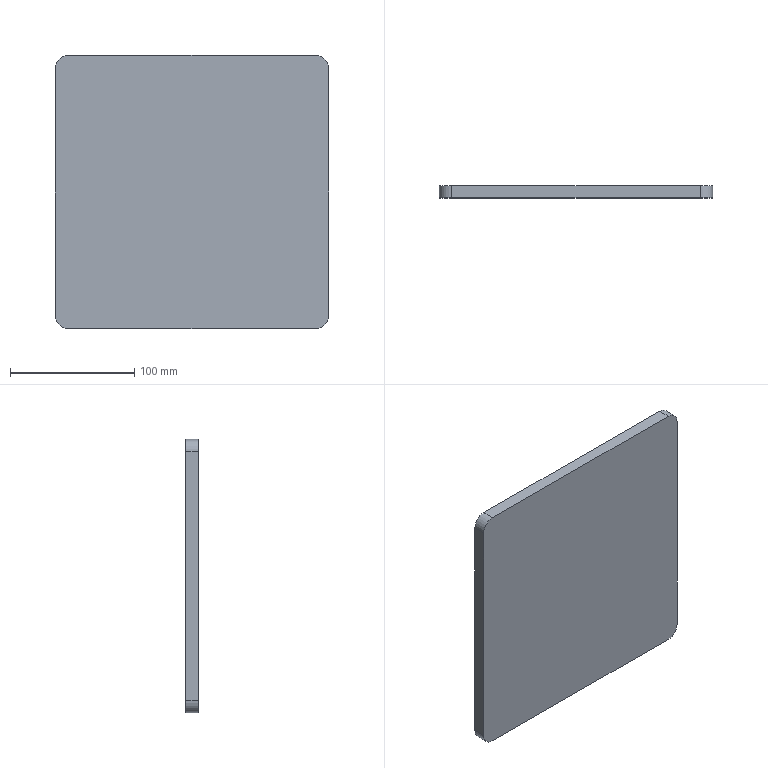Part | SolidWorks | features Extrusion 1, Fillet 1 | 1 solid | 10 faces | box 220 x 10 x 220 mm | volume 483142 mm3 | plane 6 | cylinder 4 | commonest cylinder face diameters 20 x4
STEP:
#1=CARTESIAN_POINT('',(-110.,5.,-100.));
#2=VERTEX_POINT('',#1);
#3=CARTESIAN_POINT('',(-110.,5.,100.));
#4=VERTEX_POINT('',#3);
#5=CARTESIAN_POINT('',(-110.,5.,110.));
#6=DIRECTION('',(0.,0.,1.));
#7=VECTOR('',#6,1000.);
#8=LINE('',#5,#7);
#9=EDGE_CURVE('',#2,#4,#8,.T.);
#10=ORIENTED_EDGE('',*,*,#9,.F.);
#11=CARTESIAN_POINT('',(-110.,-5.,-100.));
#12=VERTEX_POINT('',#11);
#13=CARTESIAN_POINT('',(-110.,5.,-100.));
#14=DIRECTION('',(0.,-1.,0.));
#15=VECTOR('',#14,1000.);
#16=LINE('',#13,#15);
#17=EDGE_CURVE('',#2,#12,#16,.T.);
#18=ORIENTED_EDGE('',*,*,#17,.T.);
#19=CARTESIAN_POINT('',(-110.,-5.,100.));
#20=VERTEX_POINT('',#19);
#21=CARTESIAN_POINT('',(-110.,-5.,110.));
#22=DIRECTION('',(0.,0.,1.));
#23=VECTOR('',#22,1000.);
#24=LINE('',#21,#23);
#25=EDGE_CURVE('',#12,#20,#24,.T.);
#26=ORIENTED_EDGE('',*,*,#25,.T.);
#27=CARTESIAN_POINT('',(-110.,5.,100.));
#28=DIRECTION('',(0.,1.,0.));
#29=VECTOR('',#28,1000.);
#30=LINE('',#27,#29);
#31=EDGE_CURVE('',#20,#4,#30,.T.);
#32=ORIENTED_EDGE('',*,*,#31,.T.);
#33=EDGE_LOOP('',(#10,#18,#26,#32));
#34=FACE_OUTER_BOUND('',#33,.T.);
#35=CARTESIAN_POINT('',(-110.,5.,110.));
#36=DIRECTION('',(1.,0.,0.));
#37=DIRECTION('',(0.,0.,-1.));
#38=AXIS2_PLACEMENT_3D('',#35,#36,#37);
#39=PLANE('',#38);
#40=ADVANCED_FACE('',(#34),#39,.F.);
#41=CARTESIAN_POINT('',(-100.,5.,110.));
#42=VERTEX_POINT('',#41);
#43=CARTESIAN_POINT('',(100.,5.,110.));
#44=VERTEX_POINT('',#43);
#45=CARTESIAN_POINT('',(110.,5.,110.));
#46=DIRECTION('',(1.,0.,0.));
#47=VECTOR('',#46,1000.);
#48=LINE('',#45,#47);
#49=EDGE_CURVE('',#42,#44,#48,.T.);
#50=ORIENTED_EDGE('',*,*,#49,.F.);
#51=CARTESIAN_POINT('',(-100.,-5.,110.));
#52=VERTEX_POINT('',#51);
#53=CARTESIAN_POINT('',(-100.,5.,110.));
#54=DIRECTION('',(0.,-1.,0.));
#55=VECTOR('',#54,1000.);
#56=LINE('',#53,#55);
#57=EDGE_CURVE('',#42,#52,#56,.T.);
#58=ORIENTED_EDGE('',*,*,#57,.T.);
#59=CARTESIAN_POINT('',(100.,-5.,110.));
#60=VERTEX_POINT('',#59);
#61=CARTESIAN_POINT('',(110.,-5.,110.));
#62=DIRECTION('',(1.,0.,0.));
#63=VECTOR('',#62,1000.);
#64=LINE('',#61,#63);
#65=EDGE_CURVE('',#52,#60,#64,.T.);
#66=ORIENTED_EDGE('',*,*,#65,.T.);
#67=CARTESIAN_POINT('',(100.,5.,110.));
#68=DIRECTION('',(0.,1.,0.));
#69=VECTOR('',#68,1000.);
#70=LINE('',#67,#69);
#71=EDGE_CURVE('',#60,#44,#70,.T.);
#72=ORIENTED_EDGE('',*,*,#71,.T.);
#73=EDGE_LOOP('',(#50,#58,#66,#72));
#74=FACE_OUTER_BOUND('',#73,.T.);
#75=CARTESIAN_POINT('',(110.,5.,110.));
#76=DIRECTION('',(0.,0.,-1.));
#77=DIRECTION('',(-1.,0.,0.));
#78=AXIS2_PLACEMENT_3D('',#75,#76,#77);
#79=PLANE('',#78);
#80=ADVANCED_FACE('',(#74),#79,.F.);
#81=CARTESIAN_POINT('',(110.,5.,100.));
#82=VERTEX_POINT('',#81);
#83=CARTESIAN_POINT('',(110.,5.,-100.));
#84=VERTEX_POINT('',#83);
#85=CARTESIAN_POINT('',(110.,5.,110.));
#86=DIRECTION('',(0.,0.,-1.));
#87=VECTOR('',#86,1000.);
#88=LINE('',#85,#87);
#89=EDGE_CURVE('',#82,#84,#88,.T.);
#90=ORIENTED_EDGE('',*,*,#89,.F.);
#91=CARTESIAN_POINT('',(110.,-5.,100.));
#92=VERTEX_POINT('',#91);
#93=CARTESIAN_POINT('',(110.,5.,100.));
#94=DIRECTION('',(0.,-1.,0.));
#95=VECTOR('',#94,1000.);
#96=LINE('',#93,#95);
#97=EDGE_CURVE('',#82,#92,#96,.T.);
#98=ORIENTED_EDGE('',*,*,#97,.T.);
#99=CARTESIAN_POINT('',(110.,-5.,-100.));
#100=VERTEX_POINT('',#99);
#101=CARTESIAN_POINT('',(110.,-5.,110.));
#102=DIRECTION('',(0.,0.,-1.));
#103=VECTOR('',#102,1000.);
#104=LINE('',#101,#103);
#105=EDGE_CURVE('',#92,#100,#104,.T.);
#106=ORIENTED_EDGE('',*,*,#105,.T.);
#107=CARTESIAN_POINT('',(110.,5.,-100.));
#108=DIRECTION('',(0.,1.,0.));
#109=VECTOR('',#108,1000.);
#110=LINE('',#107,#109);
#111=EDGE_CURVE('',#100,#84,#110,.T.);
#112=ORIENTED_EDGE('',*,*,#111,.T.);
#113=EDGE_LOOP('',(#90,#98,#106,#112));
#114=FACE_OUTER_BOUND('',#113,.T.);
#115=CARTESIAN_POINT('',(110.,5.,110.));
#116=DIRECTION('',(-1.,0.,0.));
#117=DIRECTION('',(0.,0.,1.));
#118=AXIS2_PLACEMENT_3D('',#115,#116,#117);
#119=PLANE('',#118);
#120=ADVANCED_FACE('',(#114),#119,.F.);
#121=CARTESIAN_POINT('',(100.,-5.,-110.));
#122=VERTEX_POINT('',#121);
#123=CARTESIAN_POINT('',(-100.,-5.,-110.));
#124=VERTEX_POINT('',#123);
#125=CARTESIAN_POINT('',(110.,-5.,-110.));
#126=DIRECTION('',(-1.,0.,0.));
#127=VECTOR('',#126,1000.);
#128=LINE('',#125,#127);
#129=EDGE_CURVE('',#122,#124,#128,.T.);
#130=ORIENTED_EDGE('',*,*,#129,.T.);
#131=CARTESIAN_POINT('',(-100.,5.,-110.));
#132=VERTEX_POINT('',#131);
#133=CARTESIAN_POINT('',(-100.,5.,-110.));
#134=DIRECTION('',(0.,1.,0.));
#135=VECTOR('',#134,1000.);
#136=LINE('',#133,#135);
#137=EDGE_CURVE('',#124,#132,#136,.T.);
#138=ORIENTED_EDGE('',*,*,#137,.T.);
#139=CARTESIAN_POINT('',(100.,5.,-110.));
#140=VERTEX_POINT('',#139);
#141=CARTESIAN_POINT('',(110.,5.,-110.));
#142=DIRECTION('',(-1.,0.,0.));
#143=VECTOR('',#142,1000.);
#144=LINE('',#141,#143);
#145=EDGE_CURVE('',#140,#132,#144,.T.);
#146=ORIENTED_EDGE('',*,*,#145,.F.);
#147=CARTESIAN_POINT('',(100.,5.,-110.));
#148=DIRECTION('',(0.,-1.,0.));
#149=VECTOR('',#148,1000.);
#150=LINE('',#147,#149);
#151=EDGE_CURVE('',#140,#122,#150,.T.);
#152=ORIENTED_EDGE('',*,*,#151,.T.);
#153=EDGE_LOOP('',(#130,#138,#146,#152));
#154=FACE_OUTER_BOUND('',#153,.T.);
#155=CARTESIAN_POINT('',(110.,5.,-110.));
#156=DIRECTION('',(0.,0.,1.));
#157=DIRECTION('',(1.,0.,0.));
#158=AXIS2_PLACEMENT_3D('',#155,#156,#157);
#159=PLANE('',#158);
#160=ADVANCED_FACE('',(#154),#159,.F.);
#161=ORIENTED_EDGE('',*,*,#145,.T.);
#162=CARTESIAN_POINT('',(-100.,5.,-100.));
#163=DIRECTION('',(0.,1.,0.));
#164=DIRECTION('',(0.,0.,1.));
#165=AXIS2_PLACEMENT_3D('',#162,#163,#164);
#166=CIRCLE('',#165,10.);
#167=EDGE_CURVE('',#132,#2,#166,.T.);
#168=ORIENTED_EDGE('',*,*,#167,.T.);
#169=ORIENTED_EDGE('',*,*,#9,.T.);
#170=CARTESIAN_POINT('',(-100.,5.,100.));
#171=DIRECTION('',(0.,1.,0.));
#172=DIRECTION('',(0.,0.,1.));
#173=AXIS2_PLACEMENT_3D('',#170,#171,#172);
#174=CIRCLE('',#173,10.);
#175=EDGE_CURVE('',#4,#42,#174,.T.);
#176=ORIENTED_EDGE('',*,*,#175,.T.);
#177=ORIENTED_EDGE('',*,*,#49,.T.);
#178=CARTESIAN_POINT('',(100.,5.,100.));
#179=DIRECTION('',(0.,1.,0.));
#180=DIRECTION('',(0.,0.,1.));
#181=AXIS2_PLACEMENT_3D('',#178,#179,#180);
#182=CIRCLE('',#181,10.);
#183=EDGE_CURVE('',#44,#82,#182,.T.);
#184=ORIENTED_EDGE('',*,*,#183,.T.);
#185=ORIENTED_EDGE('',*,*,#89,.T.);
#186=CARTESIAN_POINT('',(100.,5.,-100.));
#187=DIRECTION('',(0.,1.,0.));
#188=DIRECTION('',(0.,0.,1.));
#189=AXIS2_PLACEMENT_3D('',#186,#187,#188);
#190=CIRCLE('',#189,10.);
#191=EDGE_CURVE('',#84,#140,#190,.T.);
#192=ORIENTED_EDGE('',*,*,#191,.T.);
#193=EDGE_LOOP('',(#161,#168,#169,#176,#177,#184,#185,#192));
#194=FACE_OUTER_BOUND('',#193,.T.);
#195=CARTESIAN_POINT('',(0.,5.,0.));
#196=DIRECTION('',(0.,1.,0.));
#197=DIRECTION('',(0.,0.,1.));
#198=AXIS2_PLACEMENT_3D('',#195,#196,#197);
#199=PLANE('',#198);
#200=ADVANCED_FACE('',(#194),#199,.T.);
#201=ORIENTED_EDGE('',*,*,#25,.F.);
#202=CARTESIAN_POINT('',(-100.,-5.,-100.));
#203=DIRECTION('',(0.,-1.,0.));
#204=DIRECTION('',(0.,0.,1.));
#205=AXIS2_PLACEMENT_3D('',#202,#203,#204);
#206=CIRCLE('',#205,10.);
#207=EDGE_CURVE('',#12,#124,#206,.T.);
#208=ORIENTED_EDGE('',*,*,#207,.T.);
#209=ORIENTED_EDGE('',*,*,#129,.F.);
#210=CARTESIAN_POINT('',(100.,-5.,-100.));
#211=DIRECTION('',(0.,-1.,0.));
#212=DIRECTION('',(0.,0.,1.));
#213=AXIS2_PLACEMENT_3D('',#210,#211,#212);
#214=CIRCLE('',#213,10.);
#215=EDGE_CURVE('',#122,#100,#214,.T.);
#216=ORIENTED_EDGE('',*,*,#215,.T.);
#217=ORIENTED_EDGE('',*,*,#105,.F.);
#218=CARTESIAN_POINT('',(100.,-5.,100.));
#219=DIRECTION('',(0.,-1.,0.));
#220=DIRECTION('',(0.,0.,1.));
#221=AXIS2_PLACEMENT_3D('',#218,#219,#220);
#222=CIRCLE('',#221,10.);
#223=EDGE_CURVE('',#92,#60,#222,.T.);
#224=ORIENTED_EDGE('',*,*,#223,.T.);
#225=ORIENTED_EDGE('',*,*,#65,.F.);
#226=CARTESIAN_POINT('',(-100.,-5.,100.));
#227=DIRECTION('',(0.,-1.,0.));
#228=DIRECTION('',(0.,0.,1.));
#229=AXIS2_PLACEMENT_3D('',#226,#227,#228);
#230=CIRCLE('',#229,10.);
#231=EDGE_CURVE('',#52,#20,#230,.T.);
#232=ORIENTED_EDGE('',*,*,#231,.T.);
#233=EDGE_LOOP('',(#201,#208,#209,#216,#217,#224,#225,#232));
#234=FACE_OUTER_BOUND('',#233,.T.);
#235=CARTESIAN_POINT('',(0.,-5.,0.));
#236=DIRECTION('',(0.,1.,0.));
#237=DIRECTION('',(0.,0.,1.));
#238=AXIS2_PLACEMENT_3D('',#235,#236,#237);
#239=PLANE('',#238);
#240=ADVANCED_FACE('',(#234),#239,.F.);
#241=ORIENTED_EDGE('',*,*,#167,.F.);
#242=ORIENTED_EDGE('',*,*,#137,.F.);
#243=ORIENTED_EDGE('',*,*,#207,.F.);
#244=ORIENTED_EDGE('',*,*,#17,.F.);
#245=EDGE_LOOP('',(#241,#242,#243,#244));
#246=FACE_OUTER_BOUND('',#245,.T.);
#247=CARTESIAN_POINT('',(-100.,5.,-100.));
#248=DIRECTION('',(0.,-1.,0.));
#249=DIRECTION('',(0.,0.,-1.));
#250=AXIS2_PLACEMENT_3D('',#247,#248,#249);
#251=CYLINDRICAL_SURFACE('',#250,10.);
#252=ADVANCED_FACE('',(#246),#251,.T.);
#253=ORIENTED_EDGE('',*,*,#175,.F.);
#254=ORIENTED_EDGE('',*,*,#31,.F.);
#255=ORIENTED_EDGE('',*,*,#231,.F.);
#256=ORIENTED_EDGE('',*,*,#57,.F.);
#257=EDGE_LOOP('',(#253,#254,#255,#256));
#258=FACE_OUTER_BOUND('',#257,.T.);
#259=CARTESIAN_POINT('',(-100.,5.,100.));
#260=DIRECTION('',(0.,-1.,0.));
#261=DIRECTION('',(0.,0.,-1.));
#262=AXIS2_PLACEMENT_3D('',#259,#260,#261);
#263=CYLINDRICAL_SURFACE('',#262,10.);
#264=ADVANCED_FACE('',(#258),#263,.T.);
#265=ORIENTED_EDGE('',*,*,#183,.F.);
#266=ORIENTED_EDGE('',*,*,#71,.F.);
#267=ORIENTED_EDGE('',*,*,#223,.F.);
#268=ORIENTED_EDGE('',*,*,#97,.F.);
#269=EDGE_LOOP('',(#265,#266,#267,#268));
#270=FACE_OUTER_BOUND('',#269,.T.);
#271=CARTESIAN_POINT('',(100.,5.,100.));
#272=DIRECTION('',(0.,-1.,0.));
#273=DIRECTION('',(0.,0.,-1.));
#274=AXIS2_PLACEMENT_3D('',#271,#272,#273);
#275=CYLINDRICAL_SURFACE('',#274,10.);
#276=ADVANCED_FACE('',(#270),#275,.T.);
#277=ORIENTED_EDGE('',*,*,#191,.F.);
#278=ORIENTED_EDGE('',*,*,#111,.F.);
#279=ORIENTED_EDGE('',*,*,#215,.F.);
#280=ORIENTED_EDGE('',*,*,#151,.F.);
#281=EDGE_LOOP('',(#277,#278,#279,#280));
#282=FACE_OUTER_BOUND('',#281,.T.);
#283=CARTESIAN_POINT('',(100.,5.,-100.));
#284=DIRECTION('',(0.,-1.,0.));
#285=DIRECTION('',(0.,0.,-1.));
#286=AXIS2_PLACEMENT_3D('',#283,#284,#285);
#287=CYLINDRICAL_SURFACE('',#286,10.);
#288=ADVANCED_FACE('',(#282),#287,.T.);
#289=CLOSED_SHELL('',(#40,#80,#120,#160,#200,#240,#252,#264,#276,#288));
#290=MANIFOLD_SOLID_BREP('',#289);
#291=CARTESIAN_POINT('',(0.,0.,0.));
#292=DIRECTION('',(0.,0.,1.));
#293=DIRECTION('',(1.,0.,0.));
#294=AXIS2_PLACEMENT_3D('',#291,#292,#293);
#295=(LENGTH_UNIT()NAMED_UNIT(*)SI_UNIT(.MILLI.,.METRE.));
#296=UNCERTAINTY_MEASURE_WITH_UNIT(LENGTH_MEASURE(0.00001),#295,'','');
#297=(NAMED_UNIT(*)PLANE_ANGLE_UNIT()SI_UNIT($,.RADIAN.));
#298=(NAMED_UNIT(*)SI_UNIT($,.STERADIAN.)SOLID_ANGLE_UNIT());
#299=(GEOMETRIC_REPRESENTATION_CONTEXT(3)GLOBAL_UNCERTAINTY_ASSIGNED_CONTEXT((#296))GLOBAL_UNIT_ASSIGNED_CONTEXT((#295,#297,#298))REPRESENTATION_CONTEXT('',''));
#300=ADVANCED_BREP_SHAPE_REPRESENTATION('',(#290,#294),#299);